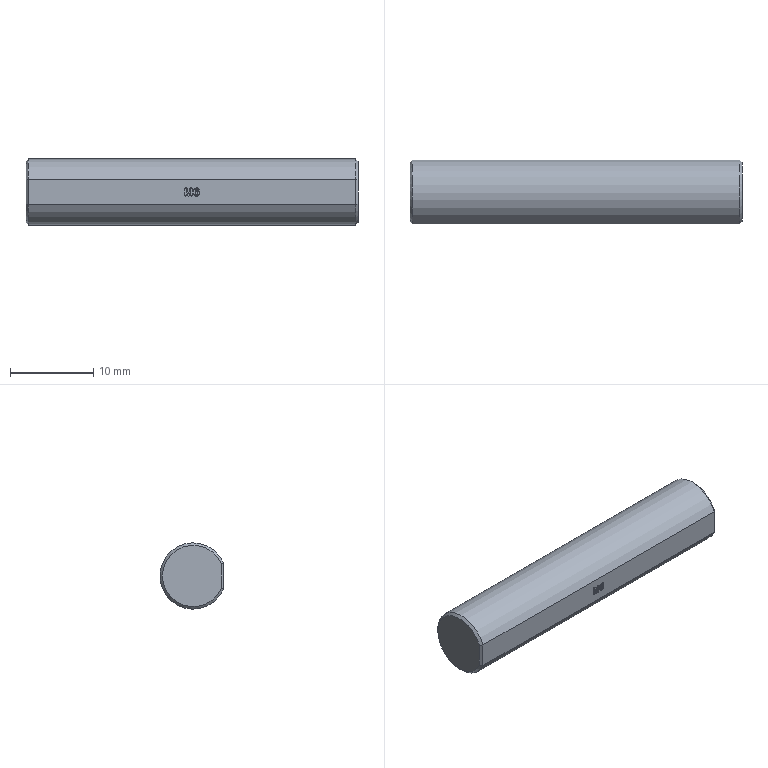Part | NX | features BREP 2, solid 2, SUBTRACT 1 | 1 solid | 28 faces | box 40 x 7.7 x 8 mm | volume 1857 mm3 | plane 12 | spline 9 | cone 4 | cylinder 3 | commonest cylinder face diameters 3.2 x1 4 x1 8 x1
STEP:
#1=CARTESIAN_POINT('',(236.55,-283.7,226.002));
#2=VERTEX_POINT('',#1);
#3=CARTESIAN_POINT('',(236.375,-283.7,226.545));
#4=VERTEX_POINT('',#3);
#5=CARTESIAN_POINT('',(236.55,-283.7,226.002));
#6=CARTESIAN_POINT('',(236.615,-283.7,226.002));
#7=CARTESIAN_POINT('',(236.673,-283.7,226.016));
#8=CARTESIAN_POINT('',(236.775,-283.7,226.073));
#9=CARTESIAN_POINT('',(236.815,-283.7,226.113));
#10=CARTESIAN_POINT('',(236.872,-283.7,226.215));
#11=CARTESIAN_POINT('',(236.886,-283.7,226.272));
#12=CARTESIAN_POINT('',(236.886,-283.7,226.377));
#13=CARTESIAN_POINT('',(236.879,-283.7,226.418));
#14=CARTESIAN_POINT('',(236.85,-283.7,226.497));
#15=CARTESIAN_POINT('',(236.829,-283.7,226.531));
#16=CARTESIAN_POINT('',(236.776,-283.7,226.589));
#17=CARTESIAN_POINT('',(236.744,-283.7,226.611));
#18=CARTESIAN_POINT('',(236.673,-283.7,226.643));
#19=CARTESIAN_POINT('',(236.634,-283.7,226.651));
#20=CARTESIAN_POINT('',(236.548,-283.7,226.651));
#21=CARTESIAN_POINT('',(236.509,-283.7,226.642));
#22=CARTESIAN_POINT('',(236.438,-283.7,226.608));
#23=CARTESIAN_POINT('',(236.405,-283.7,226.581));
#24=CARTESIAN_POINT('',(236.375,-283.7,226.545));
#25=B_SPLINE_CURVE_WITH_KNOTS('',3,(#5,#6,#7,#8,#9,#10,#11,#12,#13,#14,#15,#16,#17,#18,#19,#20,#21,#22,#23,#24),.UNSPECIFIED.,.F.,.F.,(4,2,2,2,2,2,2,2,2,4),(0.,0.02844,0.05688,0.08532,0.1049,0.1245,0.144,0.1636,0.184,0.2044),.UNSPECIFIED.);
#26=EDGE_CURVE('',#2,#4,#25,.T.);
#27=ORIENTED_EDGE('',*,*,#26,.F.);
#28=CARTESIAN_POINT('',(236.686,-283.7,226.783));
#29=VERTEX_POINT('',#28);
#30=CARTESIAN_POINT('',(236.686,-283.7,226.783));
#31=CARTESIAN_POINT('',(236.694,-283.7,226.762));
#32=CARTESIAN_POINT('',(236.706,-283.7,226.746));
#33=CARTESIAN_POINT('',(236.738,-283.7,226.722));
#34=CARTESIAN_POINT('',(236.755,-283.7,226.716));
#35=CARTESIAN_POINT('',(236.795,-283.7,226.716));
#36=CARTESIAN_POINT('',(236.812,-283.7,226.724));
#37=CARTESIAN_POINT('',(236.84,-283.7,226.754));
#38=CARTESIAN_POINT('',(236.846,-283.7,226.77));
#39=CARTESIAN_POINT('',(236.846,-283.7,226.818));
#40=CARTESIAN_POINT('',(236.836,-283.7,226.85));
#41=CARTESIAN_POINT('',(236.792,-283.7,226.915));
#42=CARTESIAN_POINT('',(236.759,-283.7,226.943));
#43=CARTESIAN_POINT('',(236.673,-283.7,226.987));
#44=CARTESIAN_POINT('',(236.623,-283.7,226.998));
#45=CARTESIAN_POINT('',(236.507,-283.7,226.998));
#46=CARTESIAN_POINT('',(236.455,-283.7,226.987));
#47=CARTESIAN_POINT('',(236.363,-283.7,226.943));
#48=CARTESIAN_POINT('',(236.324,-283.7,226.91));
#49=CARTESIAN_POINT('',(236.259,-283.7,226.823));
#50=CARTESIAN_POINT('',(236.234,-283.7,226.769));
#51=CARTESIAN_POINT('',(236.2,-283.7,226.637));
#52=CARTESIAN_POINT('',(236.191,-283.7,226.562));
#53=CARTESIAN_POINT('',(236.191,-283.7,226.375));
#54=CARTESIAN_POINT('',(236.205,-283.7,226.288));
#55=CARTESIAN_POINT('',(236.262,-283.7,226.146));
#56=CARTESIAN_POINT('',(236.304,-283.7,226.093));
#57=CARTESIAN_POINT('',(236.412,-283.7,226.02));
#58=CARTESIAN_POINT('',(236.476,-283.7,226.002));
#59=CARTESIAN_POINT('',(236.55,-283.7,226.002));
#60=B_SPLINE_CURVE_WITH_KNOTS('',3,(#30,#31,#32,#33,#34,#35,#36,#37,#38,#39,#40,#41,#42,#43,#44,#45,#46,#47,#48,#49,#50,#51,#52,#53,#54,#55,#56,#57,#58,#59),.UNSPECIFIED.,.F.,.F.,(4,2,2,2,2,2,2,2,2,2,2,2,2,2,4),(0.3727,0.3977,0.4227,0.4513,0.4798,0.5272,0.5745,0.6219,0.6711,0.7203,0.7695,0.8188,0.8792,0.9396,1.),.UNSPECIFIED.);
#61=EDGE_CURVE('',#29,#2,#60,.T.);
#62=ORIENTED_EDGE('',*,*,#61,.F.);
#63=CARTESIAN_POINT('',(236.432,-283.7,226.796));
#64=VERTEX_POINT('',#63);
#65=CARTESIAN_POINT('',(236.432,-283.7,226.796));
#66=CARTESIAN_POINT('',(236.448,-283.7,226.819));
#67=CARTESIAN_POINT('',(236.468,-283.7,226.837));
#68=CARTESIAN_POINT('',(236.514,-283.7,226.864));
#69=CARTESIAN_POINT('',(236.537,-283.7,226.871));
#70=CARTESIAN_POINT('',(236.59,-283.7,226.871));
#71=CARTESIAN_POINT('',(236.616,-283.7,226.863));
#72=CARTESIAN_POINT('',(236.66,-283.7,226.831));
#73=CARTESIAN_POINT('',(236.676,-283.7,226.809));
#74=CARTESIAN_POINT('',(236.686,-283.7,226.783));
#75=B_SPLINE_CURVE_WITH_KNOTS('',3,(#65,#66,#67,#68,#69,#70,#71,#72,#73,#74),.UNSPECIFIED.,.F.,.F.,(4,2,2,2,4),(0.2569,0.2827,0.3085,0.3406,0.3727),.UNSPECIFIED.);
#76=EDGE_CURVE('',#64,#29,#75,.T.);
#77=ORIENTED_EDGE('',*,*,#76,.F.);
#78=CARTESIAN_POINT('',(236.375,-283.7,226.545));
#79=CARTESIAN_POINT('',(236.381,-283.7,226.666));
#80=CARTESIAN_POINT('',(236.4,-283.7,226.749));
#81=CARTESIAN_POINT('',(236.432,-283.7,226.796));
#82=B_SPLINE_CURVE_WITH_KNOTS('',3,(#78,#79,#80,#81),.UNSPECIFIED.,.F.,.F.,(4,4),(0.2044,0.2569),.PIECEWISE_BEZIER_KNOTS.);
#83=EDGE_CURVE('',#4,#64,#82,.T.);
#84=ORIENTED_EDGE('',*,*,#83,.F.);
#85=EDGE_LOOP('',(#27,#62,#77,#84));
#86=FACE_BOUND('',#85,.T.);
#87=CARTESIAN_POINT('',(255.7,-283.7,228.02));
#88=VERTEX_POINT('',#87);
#89=CARTESIAN_POINT('',(216.3,-283.7,228.02));
#90=VERTEX_POINT('',#89);
#91=CARTESIAN_POINT('',(216.,-283.7,228.02));
#92=DIRECTION('',(1.,0.,0.));
#93=VECTOR('',#92,1000.);
#94=LINE('',#91,#93);
#95=EDGE_CURVE('',#88,#90,#94,.F.);
#96=ORIENTED_EDGE('',*,*,#95,.T.);
#97=CARTESIAN_POINT('',(216.3,-283.7,224.98));
#98=VERTEX_POINT('',#97);
#99=CARTESIAN_POINT('',(216.3,-283.7,224.98));
#100=DIRECTION('',(0.,0.,-1.));
#101=VECTOR('',#100,1000.);
#102=LINE('',#99,#101);
#103=EDGE_CURVE('',#90,#98,#102,.T.);
#104=ORIENTED_EDGE('',*,*,#103,.T.);
#105=CARTESIAN_POINT('',(255.7,-283.7,224.98));
#106=VERTEX_POINT('',#105);
#107=CARTESIAN_POINT('',(216.,-283.7,224.98));
#108=DIRECTION('',(1.,0.,0.));
#109=VECTOR('',#108,1000.);
#110=LINE('',#107,#109);
#111=EDGE_CURVE('',#98,#106,#110,.T.);
#112=ORIENTED_EDGE('',*,*,#111,.T.);
#113=CARTESIAN_POINT('',(255.7,-283.7,228.02));
#114=DIRECTION('',(0.,0.,1.));
#115=VECTOR('',#114,1000.);
#116=LINE('',#113,#115);
#117=EDGE_CURVE('',#106,#88,#116,.T.);
#118=ORIENTED_EDGE('',*,*,#117,.T.);
#119=EDGE_LOOP('',(#96,#104,#112,#118));
#120=FACE_BOUND('',#119,.T.);
#121=CARTESIAN_POINT('',(235.203,-283.7,226.005));
#122=VERTEX_POINT('',#121);
#123=CARTESIAN_POINT('',(235.294,-283.7,226.783));
#124=VERTEX_POINT('',#123);
#125=CARTESIAN_POINT('',(235.203,-283.7,226.005));
#126=CARTESIAN_POINT('',(235.231,-283.7,226.005));
#127=CARTESIAN_POINT('',(235.252,-283.7,226.014));
#128=CARTESIAN_POINT('',(235.285,-283.7,226.051));
#129=CARTESIAN_POINT('',(235.294,-283.7,226.079));
#130=CARTESIAN_POINT('',(235.294,-283.7,226.338));
#131=CARTESIAN_POINT('',(235.294,-283.7,226.561));
#132=CARTESIAN_POINT('',(235.294,-283.7,226.783));
#133=B_SPLINE_CURVE_WITH_KNOTS('',3,(#125,#126,#127,#128,#129,#130,#131,#132),.UNSPECIFIED.,.F.,.F.,(4,2,2,4),(0.,0.01767,0.03533,0.1418),.UNSPECIFIED.);
#134=EDGE_CURVE('',#122,#124,#133,.T.);
#135=ORIENTED_EDGE('',*,*,#134,.F.);
#136=CARTESIAN_POINT('',(235.439,-283.7,226.859));
#137=VERTEX_POINT('',#136);
#138=CARTESIAN_POINT('',(235.439,-283.7,226.859));
#139=CARTESIAN_POINT('',(235.429,-283.7,226.898));
#140=CARTESIAN_POINT('',(235.42,-283.7,226.925));
#141=CARTESIAN_POINT('',(235.404,-283.7,226.96));
#142=CARTESIAN_POINT('',(235.392,-283.7,226.972));
#143=CARTESIAN_POINT('',(235.359,-283.7,226.985));
#144=CARTESIAN_POINT('',(235.333,-283.7,226.988));
#145=CARTESIAN_POINT('',(235.276,-283.7,226.988));
#146=CARTESIAN_POINT('',(235.256,-283.7,226.988));
#147=CARTESIAN_POINT('',(235.198,-283.7,226.988));
#148=CARTESIAN_POINT('',(235.169,-283.7,226.981));
#149=CARTESIAN_POINT('',(235.125,-283.7,226.951));
#150=CARTESIAN_POINT('',(235.114,-283.7,226.923));
#151=CARTESIAN_POINT('',(235.114,-283.7,226.626));
#152=CARTESIAN_POINT('',(235.114,-283.7,226.371));
#153=CARTESIAN_POINT('',(235.114,-283.7,226.079));
#154=CARTESIAN_POINT('',(235.122,-283.7,226.051));
#155=CARTESIAN_POINT('',(235.155,-283.7,226.014));
#156=CARTESIAN_POINT('',(235.177,-283.7,226.005));
#157=CARTESIAN_POINT('',(235.203,-283.7,226.005));
#158=B_SPLINE_CURVE_WITH_KNOTS('',3,(#138,#139,#140,#141,#142,#143,#144,#145,#146,#147,#148,#149,#150,#151,#152,#153,#154,#155,#156,#157),.UNSPECIFIED.,.F.,.F.,(4,2,2,2,2,2,2,2,2,4),(0.8075,0.8217,0.8358,0.85,0.8578,0.8723,0.8868,0.9743,0.9872,1.),.UNSPECIFIED.);
#159=EDGE_CURVE('',#137,#122,#158,.T.);
#160=ORIENTED_EDGE('',*,*,#159,.F.);
#161=CARTESIAN_POINT('',(235.58,-283.7,226.33));
#162=VERTEX_POINT('',#161);
#163=CARTESIAN_POINT('',(233.874,-283.7,232.761));
#164=DIRECTION('',(-0.2564,0.,0.9666));
#165=VECTOR('',#164,1000.);
#166=LINE('',#163,#165);
#167=EDGE_CURVE('',#162,#137,#166,.T.);
#168=ORIENTED_EDGE('',*,*,#167,.F.);
#169=CARTESIAN_POINT('',(235.72,-283.7,226.859));
#170=VERTEX_POINT('',#169);
#171=CARTESIAN_POINT('',(234.712,-283.7,223.057));
#172=DIRECTION('',(-0.2564,0.,-0.9666));
#173=VECTOR('',#172,1000.);
#174=LINE('',#171,#173);
#175=EDGE_CURVE('',#170,#162,#174,.T.);
#176=ORIENTED_EDGE('',*,*,#175,.F.);
#177=CARTESIAN_POINT('',(235.866,-283.7,226.783));
#178=VERTEX_POINT('',#177);
#179=CARTESIAN_POINT('',(235.866,-283.7,226.783));
#180=CARTESIAN_POINT('',(235.866,-283.7,226.561));
#181=CARTESIAN_POINT('',(235.866,-283.7,226.338));
#182=CARTESIAN_POINT('',(235.866,-283.7,226.079));
#183=CARTESIAN_POINT('',(235.874,-283.7,226.051));
#184=CARTESIAN_POINT('',(235.908,-283.7,226.014));
#185=CARTESIAN_POINT('',(235.929,-283.7,226.005));
#186=CARTESIAN_POINT('',(235.982,-283.7,226.005));
#187=CARTESIAN_POINT('',(236.005,-283.7,226.014));
#188=CARTESIAN_POINT('',(236.038,-283.7,226.051));
#189=CARTESIAN_POINT('',(236.046,-283.7,226.079));
#190=CARTESIAN_POINT('',(236.046,-283.7,226.371));
#191=CARTESIAN_POINT('',(236.046,-283.7,226.626));
#192=CARTESIAN_POINT('',(236.046,-283.7,226.923));
#193=CARTESIAN_POINT('',(236.035,-283.7,226.951));
#194=CARTESIAN_POINT('',(235.991,-283.7,226.981));
#195=CARTESIAN_POINT('',(235.961,-283.7,226.988));
#196=CARTESIAN_POINT('',(235.904,-283.7,226.988));
#197=CARTESIAN_POINT('',(235.883,-283.7,226.988));
#198=CARTESIAN_POINT('',(235.827,-283.7,226.988));
#199=CARTESIAN_POINT('',(235.8,-283.7,226.985));
#200=CARTESIAN_POINT('',(235.767,-283.7,226.972));
#201=CARTESIAN_POINT('',(235.755,-283.7,226.96));
#202=CARTESIAN_POINT('',(235.739,-283.7,226.925));
#203=CARTESIAN_POINT('',(235.73,-283.7,226.898));
#204=CARTESIAN_POINT('',(235.72,-283.7,226.859));
#205=B_SPLINE_CURVE_WITH_KNOTS('',3,(#179,#180,#181,#182,#183,#184,#185,#186,#187,#188,#189,#190,#191,#192,#193,#194,#195,#196,#197,#198,#199,#200,#201,#202,#203,#204),.UNSPECIFIED.,.F.,.F.,(4,2,2,2,2,2,2,2,2,2,2,2,4),(0.3909,0.4624,0.4743,0.4862,0.4988,0.5115,0.599,0.6135,0.628,0.6359,0.65,0.6642,0.6783),.UNSPECIFIED.);
#206=EDGE_CURVE('',#178,#170,#205,.T.);
#207=ORIENTED_EDGE('',*,*,#206,.F.);
#208=CARTESIAN_POINT('',(235.711,-283.7,226.167));
#209=VERTEX_POINT('',#208);
#210=CARTESIAN_POINT('',(234.976,-283.7,223.245));
#211=DIRECTION('',(0.244,0.,0.9698));
#212=VECTOR('',#211,1000.);
#213=LINE('',#210,#212);
#214=EDGE_CURVE('',#209,#178,#213,.T.);
#215=ORIENTED_EDGE('',*,*,#214,.F.);
#216=CARTESIAN_POINT('',(235.449,-283.7,226.167));
#217=VERTEX_POINT('',#216);
#218=CARTESIAN_POINT('',(235.449,-283.7,226.167));
#219=CARTESIAN_POINT('',(235.454,-283.7,226.147));
#220=CARTESIAN_POINT('',(235.459,-283.7,226.128));
#221=CARTESIAN_POINT('',(235.469,-283.7,226.09));
#222=CARTESIAN_POINT('',(235.476,-283.7,226.073));
#223=CARTESIAN_POINT('',(235.494,-283.7,226.043));
#224=CARTESIAN_POINT('',(235.506,-283.7,226.03));
#225=CARTESIAN_POINT('',(235.538,-283.7,226.01));
#226=CARTESIAN_POINT('',(235.557,-283.7,226.005));
#227=CARTESIAN_POINT('',(235.61,-283.7,226.005));
#228=CARTESIAN_POINT('',(235.634,-283.7,226.013));
#229=CARTESIAN_POINT('',(235.668,-283.7,226.044));
#230=CARTESIAN_POINT('',(235.68,-283.7,226.061));
#231=CARTESIAN_POINT('',(235.693,-283.7,226.098));
#232=CARTESIAN_POINT('',(235.701,-283.7,226.127));
#233=CARTESIAN_POINT('',(235.711,-283.7,226.167));
#234=B_SPLINE_CURVE_WITH_KNOTS('',3,(#218,#219,#220,#221,#222,#223,#224,#225,#226,#227,#228,#229,#230,#231,#232,#233),.UNSPECIFIED.,.F.,.F.,(4,2,2,2,2,2,2,4),(0.243,0.253,0.263,0.273,0.283,0.2963,0.3096,0.3228),.UNSPECIFIED.);
#235=EDGE_CURVE('',#217,#209,#234,.T.);
#236=ORIENTED_EDGE('',*,*,#235,.F.);
#237=CARTESIAN_POINT('',(233.852,-283.7,232.512));
#238=DIRECTION('',(0.244,0.,-0.9698));
#239=VECTOR('',#238,1000.);
#240=LINE('',#237,#239);
#241=EDGE_CURVE('',#124,#217,#240,.T.);
#242=ORIENTED_EDGE('',*,*,#241,.F.);
#243=EDGE_LOOP('',(#135,#160,#168,#176,#207,#215,#236,#242));
#244=FACE_BOUND('',#243,.T.);
#245=CARTESIAN_POINT('',(216.,-283.7,228.02));
#246=DIRECTION('',(0.,-1.,0.));
#247=DIRECTION('',(-1.,0.,0.));
#248=AXIS2_PLACEMENT_3D('',#245,#246,#247);
#249=PLANE('',#248);
#250=ADVANCED_FACE('',(#86,#120,#244),#249,.T.);
#251=ORIENTED_EDGE('',*,*,#111,.F.);
#252=CARTESIAN_POINT('',(216.3,-280.,226.5));
#253=DIRECTION('',(1.,0.,0.));
#254=DIRECTION('',(0.,1.,0.));
#255=AXIS2_PLACEMENT_3D('',#252,#253,#254);
#256=CIRCLE('',#255,4.);
#257=EDGE_CURVE('',#98,#90,#256,.T.);
#258=ORIENTED_EDGE('',*,*,#257,.T.);
#259=ORIENTED_EDGE('',*,*,#95,.F.);
#260=CARTESIAN_POINT('',(255.7,-280.,226.5));
#261=DIRECTION('',(-1.,0.,0.));
#262=DIRECTION('',(0.,1.,0.));
#263=AXIS2_PLACEMENT_3D('',#260,#261,#262);
#264=CIRCLE('',#263,4.);
#265=EDGE_CURVE('',#88,#106,#264,.T.);
#266=ORIENTED_EDGE('',*,*,#265,.T.);
#267=EDGE_LOOP('',(#251,#258,#259,#266));
#268=FACE_BOUND('',#267,.T.);
#269=CARTESIAN_POINT('',(216.,-280.,226.5));
#270=DIRECTION('',(1.,0.,0.));
#271=DIRECTION('',(0.,-1.,0.));
#272=AXIS2_PLACEMENT_3D('',#269,#270,#271);
#273=CYLINDRICAL_SURFACE('',#272,4.);
#274=ADVANCED_FACE('',(#268),#273,.T.);
#275=CARTESIAN_POINT('',(216.,-283.4,227.959));
#276=VERTEX_POINT('',#275);
#277=CARTESIAN_POINT('',(216.,-283.4,225.041));
#278=VERTEX_POINT('',#277);
#279=CARTESIAN_POINT('',(216.,-280.,226.5));
#280=DIRECTION('',(-1.,0.,0.));
#281=DIRECTION('',(0.,1.,0.));
#282=AXIS2_PLACEMENT_3D('',#279,#280,#281);
#283=CIRCLE('',#282,3.7);
#284=EDGE_CURVE('',#276,#278,#283,.T.);
#285=ORIENTED_EDGE('',*,*,#284,.T.);
#286=CARTESIAN_POINT('',(216.,-283.4,228.02));
#287=DIRECTION('',(0.,0.,1.));
#288=VECTOR('',#287,1000.);
#289=LINE('',#286,#288);
#290=EDGE_CURVE('',#278,#276,#289,.T.);
#291=ORIENTED_EDGE('',*,*,#290,.T.);
#292=EDGE_LOOP('',(#285,#291));
#293=FACE_BOUND('',#292,.T.);
#294=CARTESIAN_POINT('',(216.,-280.,226.5));
#295=DIRECTION('',(1.,0.,0.));
#296=DIRECTION('',(0.,-1.,0.));
#297=AXIS2_PLACEMENT_3D('',#294,#295,#296);
#298=PLANE('',#297);
#299=ADVANCED_FACE('',(#293),#298,.F.);
#300=CARTESIAN_POINT('',(256.,-278.,226.5));
#301=VERTEX_POINT('',#300);
#302=CARTESIAN_POINT('',(256.,-280.,226.5));
#303=DIRECTION('',(1.,0.,0.));
#304=DIRECTION('',(0.,1.,0.));
#305=AXIS2_PLACEMENT_3D('',#302,#303,#304);
#306=CIRCLE('',#305,2.);
#307=EDGE_CURVE('',#301,#301,#306,.T.);
#308=ORIENTED_EDGE('',*,*,#307,.F.);
#309=EDGE_LOOP('',(#308));
#310=FACE_BOUND('',#309,.T.);
#311=CARTESIAN_POINT('',(256.,-283.4,227.959));
#312=VERTEX_POINT('',#311);
#313=CARTESIAN_POINT('',(256.,-283.4,225.041));
#314=VERTEX_POINT('',#313);
#315=CARTESIAN_POINT('',(256.,-283.4,226.5));
#316=DIRECTION('',(0.,0.,-1.));
#317=VECTOR('',#316,1000.);
#318=LINE('',#315,#317);
#319=EDGE_CURVE('',#312,#314,#318,.T.);
#320=ORIENTED_EDGE('',*,*,#319,.T.);
#321=CARTESIAN_POINT('',(256.,-280.,226.5));
#322=DIRECTION('',(1.,0.,0.));
#323=DIRECTION('',(0.,1.,0.));
#324=AXIS2_PLACEMENT_3D('',#321,#322,#323);
#325=CIRCLE('',#324,3.7);
#326=EDGE_CURVE('',#314,#312,#325,.T.);
#327=ORIENTED_EDGE('',*,*,#326,.T.);
#328=EDGE_LOOP('',(#320,#327));
#329=FACE_BOUND('',#328,.T.);
#330=CARTESIAN_POINT('',(256.,-280.,226.5));
#331=DIRECTION('',(1.,0.,0.));
#332=DIRECTION('',(0.,-1.,0.));
#333=AXIS2_PLACEMENT_3D('',#330,#331,#332);
#334=PLANE('',#333);
#335=ADVANCED_FACE('',(#310,#329),#334,.T.);
#336=CARTESIAN_POINT('',(216.,-283.4,225.041));
#337=CARTESIAN_POINT('',(216.1,-283.5,225.02));
#338=CARTESIAN_POINT('',(216.2,-283.6,225.));
#339=CARTESIAN_POINT('',(216.3,-283.7,224.98));
#340=B_SPLINE_CURVE_WITH_KNOTS('',3,(#336,#337,#338,#339),.UNSPECIFIED.,.F.,.F.,(4,4),(0.,1.),.PIECEWISE_BEZIER_KNOTS.);
#341=EDGE_CURVE('',#278,#98,#340,.T.);
#342=ORIENTED_EDGE('',*,*,#341,.F.);
#343=ORIENTED_EDGE('',*,*,#284,.F.);
#344=CARTESIAN_POINT('',(216.3,-283.7,228.02));
#345=CARTESIAN_POINT('',(216.2,-283.6,228.));
#346=CARTESIAN_POINT('',(216.1,-283.5,227.98));
#347=CARTESIAN_POINT('',(216.,-283.4,227.959));
#348=B_SPLINE_CURVE_WITH_KNOTS('',3,(#344,#345,#346,#347),.UNSPECIFIED.,.F.,.F.,(4,4),(0.,1.),.PIECEWISE_BEZIER_KNOTS.);
#349=EDGE_CURVE('',#90,#276,#348,.T.);
#350=ORIENTED_EDGE('',*,*,#349,.F.);
#351=ORIENTED_EDGE('',*,*,#257,.F.);
#352=EDGE_LOOP('',(#342,#343,#350,#351));
#353=FACE_BOUND('',#352,.T.);
#354=CARTESIAN_POINT('',(216.3,-280.,226.5));
#355=DIRECTION('',(1.,0.,0.));
#356=DIRECTION('',(0.,-1.,0.));
#357=AXIS2_PLACEMENT_3D('',#354,#355,#356);
#358=CONICAL_SURFACE('',#357,4.,0.7854);
#359=ADVANCED_FACE('',(#353),#358,.T.);
#360=ORIENTED_EDGE('',*,*,#349,.T.);
#361=ORIENTED_EDGE('',*,*,#290,.F.);
#362=ORIENTED_EDGE('',*,*,#341,.T.);
#363=ORIENTED_EDGE('',*,*,#103,.F.);
#364=EDGE_LOOP('',(#360,#361,#362,#363));
#365=FACE_BOUND('',#364,.T.);
#366=CARTESIAN_POINT('',(216.3,-283.7,228.02));
#367=DIRECTION('',(-0.7071,-0.7071,0.));
#368=DIRECTION('',(-0.7071,0.7071,0.));
#369=AXIS2_PLACEMENT_3D('',#366,#367,#368);
#370=PLANE('',#369);
#371=ADVANCED_FACE('',(#365),#370,.T.);
#372=CARTESIAN_POINT('',(255.7,-283.7,228.02));
#373=CARTESIAN_POINT('',(255.8,-283.6,228.));
#374=CARTESIAN_POINT('',(255.9,-283.5,227.98));
#375=CARTESIAN_POINT('',(256.,-283.4,227.959));
#376=B_SPLINE_CURVE_WITH_KNOTS('',3,(#372,#373,#374,#375),.UNSPECIFIED.,.F.,.F.,(4,4),(0.,1.),.PIECEWISE_BEZIER_KNOTS.);
#377=EDGE_CURVE('',#88,#312,#376,.T.);
#378=ORIENTED_EDGE('',*,*,#377,.F.);
#379=ORIENTED_EDGE('',*,*,#117,.F.);
#380=CARTESIAN_POINT('',(256.,-283.4,225.041));
#381=CARTESIAN_POINT('',(255.9,-283.5,225.02));
#382=CARTESIAN_POINT('',(255.8,-283.6,225.));
#383=CARTESIAN_POINT('',(255.7,-283.7,224.98));
#384=B_SPLINE_CURVE_WITH_KNOTS('',3,(#380,#381,#382,#383),.UNSPECIFIED.,.F.,.F.,(4,4),(0.,1.),.PIECEWISE_BEZIER_KNOTS.);
#385=EDGE_CURVE('',#314,#106,#384,.T.);
#386=ORIENTED_EDGE('',*,*,#385,.F.);
#387=ORIENTED_EDGE('',*,*,#319,.F.);
#388=EDGE_LOOP('',(#378,#379,#386,#387));
#389=FACE_BOUND('',#388,.T.);
#390=CARTESIAN_POINT('',(256.,-283.4,226.5));
#391=DIRECTION('',(-0.7071,0.7071,0.));
#392=DIRECTION('',(0.7071,0.7071,0.));
#393=AXIS2_PLACEMENT_3D('',#390,#391,#392);
#394=PLANE('',#393);
#395=ADVANCED_FACE('',(#389),#394,.F.);
#396=ORIENTED_EDGE('',*,*,#385,.T.);
#397=ORIENTED_EDGE('',*,*,#265,.F.);
#398=ORIENTED_EDGE('',*,*,#377,.T.);
#399=ORIENTED_EDGE('',*,*,#326,.F.);
#400=EDGE_LOOP('',(#396,#397,#398,#399));
#401=FACE_BOUND('',#400,.T.);
#402=CARTESIAN_POINT('',(256.,-280.,226.5));
#403=DIRECTION('',(-1.,0.,0.));
#404=DIRECTION('',(0.,1.,0.));
#405=AXIS2_PLACEMENT_3D('',#402,#403,#404);
#406=CONICAL_SURFACE('',#405,3.7,0.7854);
#407=ADVANCED_FACE('',(#401),#406,.T.);
#408=CARTESIAN_POINT('',(244.176,-280.,226.5));
#409=VERTEX_POINT('',#408);
#410=VERTEX_LOOP('',#409);
#411=FACE_BOUND('',#410,.T.);
#412=CARTESIAN_POINT('',(245.1,-278.4,226.5));
#413=VERTEX_POINT('',#412);
#414=CARTESIAN_POINT('',(245.1,-280.,226.5));
#415=DIRECTION('',(-1.,0.,0.));
#416=DIRECTION('',(0.,1.,0.));
#417=AXIS2_PLACEMENT_3D('',#414,#415,#416);
#418=CIRCLE('',#417,1.6);
#419=EDGE_CURVE('',#413,#413,#418,.T.);
#420=ORIENTED_EDGE('',*,*,#419,.F.);
#421=EDGE_LOOP('',(#420));
#422=FACE_BOUND('',#421,.T.);
#423=CARTESIAN_POINT('',(245.1,-280.,226.5));
#424=DIRECTION('',(1.,0.,0.));
#425=DIRECTION('',(0.,-1.,0.));
#426=AXIS2_PLACEMENT_3D('',#423,#424,#425);
#427=CONICAL_SURFACE('',#426,1.6,1.047);
#428=ADVANCED_FACE('',(#411,#422),#427,.F.);
#429=ORIENTED_EDGE('',*,*,#419,.T.);
#430=EDGE_LOOP('',(#429));
#431=FACE_BOUND('',#430,.T.);
#432=CARTESIAN_POINT('',(247.6,-278.4,226.5));
#433=VERTEX_POINT('',#432);
#434=CARTESIAN_POINT('',(247.6,-280.,226.5));
#435=DIRECTION('',(-1.,0.,0.));
#436=DIRECTION('',(0.,1.,0.));
#437=AXIS2_PLACEMENT_3D('',#434,#435,#436);
#438=CIRCLE('',#437,1.6);
#439=EDGE_CURVE('',#433,#433,#438,.T.);
#440=ORIENTED_EDGE('',*,*,#439,.F.);
#441=EDGE_LOOP('',(#440));
#442=FACE_BOUND('',#441,.T.);
#443=CARTESIAN_POINT('',(256.,-280.,226.5));
#444=DIRECTION('',(1.,0.,0.));
#445=DIRECTION('',(0.,-1.,0.));
#446=AXIS2_PLACEMENT_3D('',#443,#444,#445);
#447=CYLINDRICAL_SURFACE('',#446,1.6);
#448=ADVANCED_FACE('',(#431,#442),#447,.F.);
#449=ORIENTED_EDGE('',*,*,#439,.T.);
#450=EDGE_LOOP('',(#449));
#451=FACE_BOUND('',#450,.T.);
#452=CARTESIAN_POINT('',(248.,-278.,226.5));
#453=VERTEX_POINT('',#452);
#454=CARTESIAN_POINT('',(248.,-280.,226.5));
#455=DIRECTION('',(-1.,0.,0.));
#456=DIRECTION('',(0.,1.,0.));
#457=AXIS2_PLACEMENT_3D('',#454,#455,#456);
#458=CIRCLE('',#457,2.);
#459=EDGE_CURVE('',#453,#453,#458,.T.);
#460=ORIENTED_EDGE('',*,*,#459,.F.);
#461=EDGE_LOOP('',(#460));
#462=FACE_BOUND('',#461,.T.);
#463=CARTESIAN_POINT('',(248.,-280.,226.5));
#464=DIRECTION('',(1.,0.,0.));
#465=DIRECTION('',(0.,-1.,0.));
#466=AXIS2_PLACEMENT_3D('',#463,#464,#465);
#467=CONICAL_SURFACE('',#466,2.,0.7854);
#468=ADVANCED_FACE('',(#451,#462),#467,.F.);
#469=ORIENTED_EDGE('',*,*,#459,.T.);
#470=EDGE_LOOP('',(#469));
#471=FACE_BOUND('',#470,.T.);
#472=ORIENTED_EDGE('',*,*,#307,.T.);
#473=EDGE_LOOP('',(#472));
#474=FACE_BOUND('',#473,.T.);
#475=CARTESIAN_POINT('',(256.,-280.,226.5));
#476=DIRECTION('',(1.,0.,0.));
#477=DIRECTION('',(0.,-1.,0.));
#478=AXIS2_PLACEMENT_3D('',#475,#476,#477);
#479=CYLINDRICAL_SURFACE('',#478,2.);
#480=ADVANCED_FACE('',(#471,#474),#479,.F.);
#481=ORIENTED_EDGE('',*,*,#134,.T.);
#482=CARTESIAN_POINT('',(235.294,-283.5,226.783));
#483=VERTEX_POINT('',#482);
#484=CARTESIAN_POINT('',(235.294,-283.5,226.783));
#485=DIRECTION('',(0.,-1.,0.));
#486=VECTOR('',#485,1000.);
#487=LINE('',#484,#486);
#488=EDGE_CURVE('',#124,#483,#487,.F.);
#489=ORIENTED_EDGE('',*,*,#488,.T.);
#490=CARTESIAN_POINT('',(235.203,-283.5,226.005));
#491=VERTEX_POINT('',#490);
#492=CARTESIAN_POINT('',(235.203,-283.5,226.005));
#493=CARTESIAN_POINT('',(235.231,-283.5,226.005));
#494=CARTESIAN_POINT('',(235.252,-283.5,226.014));
#495=CARTESIAN_POINT('',(235.285,-283.5,226.051));
#496=CARTESIAN_POINT('',(235.294,-283.5,226.079));
#497=CARTESIAN_POINT('',(235.294,-283.5,226.338));
#498=CARTESIAN_POINT('',(235.294,-283.5,226.561));
#499=CARTESIAN_POINT('',(235.294,-283.5,226.783));
#500=B_SPLINE_CURVE_WITH_KNOTS('',3,(#492,#493,#494,#495,#496,#497,#498,#499),.UNSPECIFIED.,.F.,.F.,(4,2,2,4),(0.,0.01767,0.03533,0.1418),.UNSPECIFIED.);
#501=EDGE_CURVE('',#483,#491,#500,.F.);
#502=ORIENTED_EDGE('',*,*,#501,.T.);
#503=CARTESIAN_POINT('',(235.203,-283.5,226.005));
#504=DIRECTION('',(0.,-1.,0.));
#505=VECTOR('',#504,1000.);
#506=LINE('',#503,#505);
#507=EDGE_CURVE('',#122,#491,#506,.F.);
#508=ORIENTED_EDGE('',*,*,#507,.F.);
#509=EDGE_LOOP('',(#481,#489,#502,#508));
#510=FACE_BOUND('',#509,.T.);
#511=CARTESIAN_POINT('',(235.203,-283.5,226.005));
#512=CARTESIAN_POINT('',(235.203,-283.7,226.005));
#513=CARTESIAN_POINT('',(235.313,-283.5,226.005));
#514=CARTESIAN_POINT('',(235.313,-283.7,226.005));
#515=CARTESIAN_POINT('',(235.284,-283.5,226.357));
#516=CARTESIAN_POINT('',(235.284,-283.7,226.357));
#517=CARTESIAN_POINT('',(235.294,-283.5,226.635));
#518=CARTESIAN_POINT('',(235.294,-283.7,226.635));
#519=CARTESIAN_POINT('',(235.294,-283.5,226.783));
#520=CARTESIAN_POINT('',(235.294,-283.7,226.783));
#521=B_SPLINE_SURFACE_WITH_KNOTS('',3,1,((#511,#512),(#513,#514),(#515,#516),(#517,#518),(#519,#520)),.SURF_OF_LINEAR_EXTRUSION.,.F.,.F.,.F.,(4,1,4),(2,2),(0.,0.07088,0.1418),(0.,1.),.UNSPECIFIED.);
#522=ADVANCED_FACE('',(#510),#521,.F.);
#523=ORIENTED_EDGE('',*,*,#241,.T.);
#524=CARTESIAN_POINT('',(235.449,-283.5,226.167));
#525=VERTEX_POINT('',#524);
#526=CARTESIAN_POINT('',(235.449,-283.5,226.167));
#527=DIRECTION('',(0.,-1.,0.));
#528=VECTOR('',#527,1000.);
#529=LINE('',#526,#528);
#530=EDGE_CURVE('',#217,#525,#529,.F.);
#531=ORIENTED_EDGE('',*,*,#530,.T.);
#532=CARTESIAN_POINT('',(235.294,-283.5,226.783));
#533=CARTESIAN_POINT('',(235.345,-283.5,226.578));
#534=CARTESIAN_POINT('',(235.397,-283.5,226.373));
#535=CARTESIAN_POINT('',(235.449,-283.5,226.167));
#536=B_SPLINE_CURVE_WITH_KNOTS('',3,(#532,#533,#534,#535),.UNSPECIFIED.,.F.,.F.,(4,4),(0.1418,0.243),.PIECEWISE_BEZIER_KNOTS.);
#537=EDGE_CURVE('',#525,#483,#536,.F.);
#538=ORIENTED_EDGE('',*,*,#537,.T.);
#539=ORIENTED_EDGE('',*,*,#488,.F.);
#540=EDGE_LOOP('',(#523,#531,#538,#539));
#541=FACE_BOUND('',#540,.T.);
#542=CARTESIAN_POINT('',(235.294,-283.5,226.783));
#543=DIRECTION('',(-0.9698,0.,-0.244));
#544=DIRECTION('',(-0.244,0.,0.9698));
#545=AXIS2_PLACEMENT_3D('',#542,#543,#544);
#546=PLANE('',#545);
#547=ADVANCED_FACE('',(#541),#546,.F.);
#548=ORIENTED_EDGE('',*,*,#235,.T.);
#549=CARTESIAN_POINT('',(235.711,-283.5,226.167));
#550=VERTEX_POINT('',#549);
#551=CARTESIAN_POINT('',(235.711,-283.5,226.167));
#552=DIRECTION('',(0.,-1.,0.));
#553=VECTOR('',#552,1000.);
#554=LINE('',#551,#553);
#555=EDGE_CURVE('',#209,#550,#554,.F.);
#556=ORIENTED_EDGE('',*,*,#555,.T.);
#557=CARTESIAN_POINT('',(235.449,-283.5,226.167));
#558=CARTESIAN_POINT('',(235.454,-283.5,226.147));
#559=CARTESIAN_POINT('',(235.459,-283.5,226.128));
#560=CARTESIAN_POINT('',(235.469,-283.5,226.09));
#561=CARTESIAN_POINT('',(235.476,-283.5,226.073));
#562=CARTESIAN_POINT('',(235.494,-283.5,226.043));
#563=CARTESIAN_POINT('',(235.506,-283.5,226.03));
#564=CARTESIAN_POINT('',(235.538,-283.5,226.01));
#565=CARTESIAN_POINT('',(235.557,-283.5,226.005));
#566=CARTESIAN_POINT('',(235.61,-283.5,226.005));
#567=CARTESIAN_POINT('',(235.634,-283.5,226.013));
#568=CARTESIAN_POINT('',(235.668,-283.5,226.044));
#569=CARTESIAN_POINT('',(235.68,-283.5,226.061));
#570=CARTESIAN_POINT('',(235.693,-283.5,226.098));
#571=CARTESIAN_POINT('',(235.701,-283.5,226.127));
#572=CARTESIAN_POINT('',(235.711,-283.5,226.167));
#573=B_SPLINE_CURVE_WITH_KNOTS('',3,(#557,#558,#559,#560,#561,#562,#563,#564,#565,#566,#567,#568,#569,#570,#571,#572),.UNSPECIFIED.,.F.,.F.,(4,2,2,2,2,2,2,4),(0.243,0.253,0.263,0.273,0.283,0.2963,0.3096,0.3228),.UNSPECIFIED.);
#574=EDGE_CURVE('',#550,#525,#573,.F.);
#575=ORIENTED_EDGE('',*,*,#574,.T.);
#576=ORIENTED_EDGE('',*,*,#530,.F.);
#577=EDGE_LOOP('',(#548,#556,#575,#576));
#578=FACE_BOUND('',#577,.T.);
#579=CARTESIAN_POINT('',(235.449,-283.5,226.167));
#580=CARTESIAN_POINT('',(235.449,-283.7,226.167));
#581=CARTESIAN_POINT('',(235.491,-283.5,226.006));
#582=CARTESIAN_POINT('',(235.491,-283.7,226.006));
#583=CARTESIAN_POINT('',(235.65,-283.5,225.927));
#584=CARTESIAN_POINT('',(235.65,-283.7,225.927));
#585=CARTESIAN_POINT('',(235.711,-283.5,226.167));
#586=CARTESIAN_POINT('',(235.711,-283.7,226.167));
#587=B_SPLINE_SURFACE_WITH_KNOTS('',3,1,((#579,#580),(#581,#582),(#583,#584),(#585,#586)),.SURF_OF_LINEAR_EXTRUSION.,.F.,.F.,.F.,(4,4),(2,2),(0.243,0.3228),(0.,1.),.PIECEWISE_BEZIER_KNOTS.);
#588=ADVANCED_FACE('',(#578),#587,.F.);
#589=ORIENTED_EDGE('',*,*,#214,.T.);
#590=CARTESIAN_POINT('',(235.866,-283.5,226.783));
#591=VERTEX_POINT('',#590);
#592=CARTESIAN_POINT('',(235.866,-283.5,226.783));
#593=DIRECTION('',(0.,-1.,0.));
#594=VECTOR('',#593,1000.);
#595=LINE('',#592,#594);
#596=EDGE_CURVE('',#178,#591,#595,.F.);
#597=ORIENTED_EDGE('',*,*,#596,.T.);
#598=CARTESIAN_POINT('',(235.711,-283.5,226.167));
#599=CARTESIAN_POINT('',(235.763,-283.5,226.373));
#600=CARTESIAN_POINT('',(235.814,-283.5,226.578));
#601=CARTESIAN_POINT('',(235.866,-283.5,226.783));
#602=B_SPLINE_CURVE_WITH_KNOTS('',3,(#598,#599,#600,#601),.UNSPECIFIED.,.F.,.F.,(4,4),(0.3228,0.3909),.PIECEWISE_BEZIER_KNOTS.);
#603=EDGE_CURVE('',#591,#550,#602,.F.);
#604=ORIENTED_EDGE('',*,*,#603,.T.);
#605=ORIENTED_EDGE('',*,*,#555,.F.);
#606=EDGE_LOOP('',(#589,#597,#604,#605));
#607=FACE_BOUND('',#606,.T.);
#608=CARTESIAN_POINT('',(235.711,-283.5,226.167));
#609=DIRECTION('',(0.9698,0.,-0.244));
#610=DIRECTION('',(-0.244,0.,-0.9698));
#611=AXIS2_PLACEMENT_3D('',#608,#609,#610);
#612=PLANE('',#611);
#613=ADVANCED_FACE('',(#607),#612,.F.);
#614=ORIENTED_EDGE('',*,*,#206,.T.);
#615=CARTESIAN_POINT('',(235.72,-283.5,226.859));
#616=VERTEX_POINT('',#615);
#617=CARTESIAN_POINT('',(235.72,-283.5,226.859));
#618=DIRECTION('',(0.,-1.,0.));
#619=VECTOR('',#618,1000.);
#620=LINE('',#617,#619);
#621=EDGE_CURVE('',#170,#616,#620,.F.);
#622=ORIENTED_EDGE('',*,*,#621,.T.);
#623=CARTESIAN_POINT('',(235.866,-283.5,226.783));
#624=CARTESIAN_POINT('',(235.866,-283.5,226.561));
#625=CARTESIAN_POINT('',(235.866,-283.5,226.338));
#626=CARTESIAN_POINT('',(235.866,-283.5,226.079));
#627=CARTESIAN_POINT('',(235.874,-283.5,226.051));
#628=CARTESIAN_POINT('',(235.908,-283.5,226.014));
#629=CARTESIAN_POINT('',(235.929,-283.5,226.005));
#630=CARTESIAN_POINT('',(235.982,-283.5,226.005));
#631=CARTESIAN_POINT('',(236.005,-283.5,226.014));
#632=CARTESIAN_POINT('',(236.038,-283.5,226.051));
#633=CARTESIAN_POINT('',(236.046,-283.5,226.079));
#634=CARTESIAN_POINT('',(236.046,-283.5,226.371));
#635=CARTESIAN_POINT('',(236.046,-283.5,226.626));
#636=CARTESIAN_POINT('',(236.046,-283.5,226.923));
#637=CARTESIAN_POINT('',(236.035,-283.5,226.951));
#638=CARTESIAN_POINT('',(235.991,-283.5,226.981));
#639=CARTESIAN_POINT('',(235.961,-283.5,226.988));
#640=CARTESIAN_POINT('',(235.904,-283.5,226.988));
#641=CARTESIAN_POINT('',(235.883,-283.5,226.988));
#642=CARTESIAN_POINT('',(235.827,-283.5,226.988));
#643=CARTESIAN_POINT('',(235.8,-283.5,226.985));
#644=CARTESIAN_POINT('',(235.767,-283.5,226.972));
#645=CARTESIAN_POINT('',(235.755,-283.5,226.96));
#646=CARTESIAN_POINT('',(235.739,-283.5,226.925));
#647=CARTESIAN_POINT('',(235.73,-283.5,226.898));
#648=CARTESIAN_POINT('',(235.72,-283.5,226.859));
#649=B_SPLINE_CURVE_WITH_KNOTS('',3,(#623,#624,#625,#626,#627,#628,#629,#630,#631,#632,#633,#634,#635,#636,#637,#638,#639,#640,#641,#642,#643,#644,#645,#646,#647,#648),.UNSPECIFIED.,.F.,.F.,(4,2,2,2,2,2,2,2,2,2,2,2,4),(0.3909,0.4624,0.4743,0.4862,0.4988,0.5115,0.599,0.6135,0.628,0.6359,0.65,0.6642,0.6783),.UNSPECIFIED.);
#650=EDGE_CURVE('',#616,#591,#649,.F.);
#651=ORIENTED_EDGE('',*,*,#650,.T.);
#652=ORIENTED_EDGE('',*,*,#596,.F.);
#653=EDGE_LOOP('',(#614,#622,#651,#652));
#654=FACE_BOUND('',#653,.T.);
#655=CARTESIAN_POINT('',(235.866,-283.5,226.783));
#656=CARTESIAN_POINT('',(235.866,-283.7,226.783));
#657=CARTESIAN_POINT('',(235.866,-283.5,226.671));
#658=CARTESIAN_POINT('',(235.866,-283.7,226.671));
#659=CARTESIAN_POINT('',(235.881,-283.5,226.461));
#660=CARTESIAN_POINT('',(235.881,-283.7,226.461));
#661=CARTESIAN_POINT('',(235.812,-283.5,226.067));
#662=CARTESIAN_POINT('',(235.812,-283.7,226.067));
#663=CARTESIAN_POINT('',(236.067,-283.5,225.947));
#664=CARTESIAN_POINT('',(236.067,-283.7,225.947));
#665=CARTESIAN_POINT('',(236.044,-283.5,226.336));
#666=CARTESIAN_POINT('',(236.044,-283.7,226.336));
#667=CARTESIAN_POINT('',(236.031,-283.5,226.613));
#668=CARTESIAN_POINT('',(236.031,-283.7,226.613));
#669=CARTESIAN_POINT('',(236.106,-283.5,227.));
#670=CARTESIAN_POINT('',(236.106,-283.7,227.));
#671=CARTESIAN_POINT('',(235.769,-283.5,226.994));
#672=CARTESIAN_POINT('',(235.769,-283.7,226.994));
#673=CARTESIAN_POINT('',(235.746,-283.5,226.957));
#674=CARTESIAN_POINT('',(235.746,-283.7,226.957));
#675=CARTESIAN_POINT('',(235.72,-283.5,226.859));
#676=CARTESIAN_POINT('',(235.72,-283.7,226.859));
#677=B_SPLINE_SURFACE_WITH_KNOTS('',3,1,((#655,#656),(#657,#658),(#659,#660),(#661,#662),(#663,#664),(#665,#666),(#667,#668),(#669,#670),(#671,#672),(#673,#674),(#675,#676)),.SURF_OF_LINEAR_EXTRUSION.,.F.,.F.,.F.,(4,1,1,1,1,1,1,1,4),(2,2),(0.3909,0.4268,0.4627,0.4987,0.5346,0.5705,0.6065,0.6424,0.6783),(0.,1.),.UNSPECIFIED.);
#678=ADVANCED_FACE('',(#654),#677,.F.);
#679=ORIENTED_EDGE('',*,*,#175,.T.);
#680=CARTESIAN_POINT('',(235.58,-283.5,226.33));
#681=VERTEX_POINT('',#680);
#682=CARTESIAN_POINT('',(235.58,-283.5,226.33));
#683=DIRECTION('',(0.,-1.,0.));
#684=VECTOR('',#683,1000.);
#685=LINE('',#682,#684);
#686=EDGE_CURVE('',#162,#681,#685,.F.);
#687=ORIENTED_EDGE('',*,*,#686,.T.);
#688=CARTESIAN_POINT('',(235.72,-283.5,226.859));
#689=CARTESIAN_POINT('',(235.673,-283.5,226.682));
#690=CARTESIAN_POINT('',(235.627,-283.5,226.506));
#691=CARTESIAN_POINT('',(235.58,-283.5,226.33));
#692=B_SPLINE_CURVE_WITH_KNOTS('',3,(#688,#689,#690,#691),.UNSPECIFIED.,.F.,.F.,(4,4),(0.6783,0.7429),.PIECEWISE_BEZIER_KNOTS.);
#693=EDGE_CURVE('',#681,#616,#692,.F.);
#694=ORIENTED_EDGE('',*,*,#693,.T.);
#695=ORIENTED_EDGE('',*,*,#621,.F.);
#696=EDGE_LOOP('',(#679,#687,#694,#695));
#697=FACE_BOUND('',#696,.T.);
#698=CARTESIAN_POINT('',(235.72,-283.5,226.859));
#699=DIRECTION('',(-0.9666,0.,0.2564));
#700=DIRECTION('',(0.2564,0.,0.9666));
#701=AXIS2_PLACEMENT_3D('',#698,#699,#700);
#702=PLANE('',#701);
#703=ADVANCED_FACE('',(#697),#702,.F.);
#704=ORIENTED_EDGE('',*,*,#167,.T.);
#705=CARTESIAN_POINT('',(235.439,-283.5,226.859));
#706=VERTEX_POINT('',#705);
#707=CARTESIAN_POINT('',(235.439,-283.5,226.859));
#708=DIRECTION('',(0.,-1.,0.));
#709=VECTOR('',#708,1000.);
#710=LINE('',#707,#709);
#711=EDGE_CURVE('',#137,#706,#710,.F.);
#712=ORIENTED_EDGE('',*,*,#711,.T.);
#713=CARTESIAN_POINT('',(235.58,-283.5,226.33));
#714=CARTESIAN_POINT('',(235.533,-283.5,226.506));
#715=CARTESIAN_POINT('',(235.486,-283.5,226.682));
#716=CARTESIAN_POINT('',(235.439,-283.5,226.859));
#717=B_SPLINE_CURVE_WITH_KNOTS('',3,(#713,#714,#715,#716),.UNSPECIFIED.,.F.,.F.,(4,4),(0.7429,0.8075),.PIECEWISE_BEZIER_KNOTS.);
#718=EDGE_CURVE('',#706,#681,#717,.F.);
#719=ORIENTED_EDGE('',*,*,#718,.T.);
#720=ORIENTED_EDGE('',*,*,#686,.F.);
#721=EDGE_LOOP('',(#704,#712,#719,#720));
#722=FACE_BOUND('',#721,.T.);
#723=CARTESIAN_POINT('',(235.58,-283.5,226.33));
#724=DIRECTION('',(0.9666,0.,0.2564));
#725=DIRECTION('',(0.2564,0.,-0.9666));
#726=AXIS2_PLACEMENT_3D('',#723,#724,#725);
#727=PLANE('',#726);
#728=ADVANCED_FACE('',(#722),#727,.F.);
#729=ORIENTED_EDGE('',*,*,#159,.T.);
#730=ORIENTED_EDGE('',*,*,#507,.T.);
#731=CARTESIAN_POINT('',(235.439,-283.5,226.859));
#732=CARTESIAN_POINT('',(235.429,-283.5,226.898));
#733=CARTESIAN_POINT('',(235.42,-283.5,226.925));
#734=CARTESIAN_POINT('',(235.404,-283.5,226.96));
#735=CARTESIAN_POINT('',(235.392,-283.5,226.972));
#736=CARTESIAN_POINT('',(235.359,-283.5,226.985));
#737=CARTESIAN_POINT('',(235.333,-283.5,226.988));
#738=CARTESIAN_POINT('',(235.276,-283.5,226.988));
#739=CARTESIAN_POINT('',(235.256,-283.5,226.988));
#740=CARTESIAN_POINT('',(235.198,-283.5,226.988));
#741=CARTESIAN_POINT('',(235.169,-283.5,226.981));
#742=CARTESIAN_POINT('',(235.125,-283.5,226.951));
#743=CARTESIAN_POINT('',(235.114,-283.5,226.923));
#744=CARTESIAN_POINT('',(235.114,-283.5,226.626));
#745=CARTESIAN_POINT('',(235.114,-283.5,226.371));
#746=CARTESIAN_POINT('',(235.114,-283.5,226.079));
#747=CARTESIAN_POINT('',(235.122,-283.5,226.051));
#748=CARTESIAN_POINT('',(235.155,-283.5,226.014));
#749=CARTESIAN_POINT('',(235.177,-283.5,226.005));
#750=CARTESIAN_POINT('',(235.203,-283.5,226.005));
#751=B_SPLINE_CURVE_WITH_KNOTS('',3,(#731,#732,#733,#734,#735,#736,#737,#738,#739,#740,#741,#742,#743,#744,#745,#746,#747,#748,#749,#750),.UNSPECIFIED.,.F.,.F.,(4,2,2,2,2,2,2,2,2,4),(0.8075,0.8217,0.8358,0.85,0.8578,0.8723,0.8868,0.9743,0.9872,1.),.UNSPECIFIED.);
#752=EDGE_CURVE('',#491,#706,#751,.F.);
#753=ORIENTED_EDGE('',*,*,#752,.T.);
#754=ORIENTED_EDGE('',*,*,#711,.F.);
#755=EDGE_LOOP('',(#729,#730,#753,#754));
#756=FACE_BOUND('',#755,.T.);
#757=CARTESIAN_POINT('',(235.439,-283.5,226.859));
#758=CARTESIAN_POINT('',(235.439,-283.7,226.859));
#759=CARTESIAN_POINT('',(235.422,-283.5,226.925));
#760=CARTESIAN_POINT('',(235.422,-283.7,226.925));
#761=CARTESIAN_POINT('',(235.414,-283.5,226.984));
#762=CARTESIAN_POINT('',(235.414,-283.7,226.984));
#763=CARTESIAN_POINT('',(235.253,-283.5,226.994));
#764=CARTESIAN_POINT('',(235.253,-283.7,226.994));
#765=CARTESIAN_POINT('',(235.09,-283.5,226.969));
#766=CARTESIAN_POINT('',(235.09,-283.7,226.969));
#767=CARTESIAN_POINT('',(235.127,-283.5,226.646));
#768=CARTESIAN_POINT('',(235.127,-283.7,226.646));
#769=CARTESIAN_POINT('',(235.113,-283.5,226.33));
#770=CARTESIAN_POINT('',(235.113,-283.7,226.33));
#771=CARTESIAN_POINT('',(235.104,-283.5,226.005));
#772=CARTESIAN_POINT('',(235.104,-283.7,226.005));
#773=CARTESIAN_POINT('',(235.203,-283.5,226.005));
#774=CARTESIAN_POINT('',(235.203,-283.7,226.005));
#775=B_SPLINE_SURFACE_WITH_KNOTS('',3,1,((#757,#758),(#759,#760),(#761,#762),(#763,#764),(#765,#766),(#767,#768),(#769,#770),(#771,#772),(#773,#774)),.SURF_OF_LINEAR_EXTRUSION.,.F.,.F.,.F.,(4,1,1,1,1,1,4),(2,2),(0.8075,0.8316,0.8557,0.8797,0.9038,0.9519,1.),(0.,1.),.UNSPECIFIED.);
#776=ADVANCED_FACE('',(#756),#775,.F.);
#777=ORIENTED_EDGE('',*,*,#501,.F.);
#778=ORIENTED_EDGE('',*,*,#537,.F.);
#779=ORIENTED_EDGE('',*,*,#574,.F.);
#780=ORIENTED_EDGE('',*,*,#603,.F.);
#781=ORIENTED_EDGE('',*,*,#650,.F.);
#782=ORIENTED_EDGE('',*,*,#693,.F.);
#783=ORIENTED_EDGE('',*,*,#718,.F.);
#784=ORIENTED_EDGE('',*,*,#752,.F.);
#785=EDGE_LOOP('',(#777,#778,#779,#780,#781,#782,#783,#784));
#786=FACE_BOUND('',#785,.T.);
#787=CARTESIAN_POINT('',(235.294,-283.5,226.339));
#788=DIRECTION('',(0.,1.,0.));
#789=DIRECTION('',(0.,0.,1.));
#790=AXIS2_PLACEMENT_3D('',#787,#788,#789);
#791=PLANE('',#790);
#792=ADVANCED_FACE('',(#786),#791,.F.);
#793=ORIENTED_EDGE('',*,*,#26,.T.);
#794=CARTESIAN_POINT('',(236.375,-283.5,226.545));
#795=VERTEX_POINT('',#794);
#796=CARTESIAN_POINT('',(236.375,-283.5,226.545));
#797=DIRECTION('',(0.,-1.,0.));
#798=VECTOR('',#797,1000.);
#799=LINE('',#796,#798);
#800=EDGE_CURVE('',#4,#795,#799,.F.);
#801=ORIENTED_EDGE('',*,*,#800,.T.);
#802=CARTESIAN_POINT('',(236.55,-283.5,226.002));
#803=VERTEX_POINT('',#802);
#804=CARTESIAN_POINT('',(236.55,-283.5,226.002));
#805=CARTESIAN_POINT('',(236.615,-283.5,226.002));
#806=CARTESIAN_POINT('',(236.673,-283.5,226.016));
#807=CARTESIAN_POINT('',(236.775,-283.5,226.073));
#808=CARTESIAN_POINT('',(236.815,-283.5,226.113));
#809=CARTESIAN_POINT('',(236.872,-283.5,226.215));
#810=CARTESIAN_POINT('',(236.886,-283.5,226.272));
#811=CARTESIAN_POINT('',(236.886,-283.5,226.377));
#812=CARTESIAN_POINT('',(236.879,-283.5,226.418));
#813=CARTESIAN_POINT('',(236.85,-283.5,226.497));
#814=CARTESIAN_POINT('',(236.829,-283.5,226.531));
#815=CARTESIAN_POINT('',(236.776,-283.5,226.589));
#816=CARTESIAN_POINT('',(236.744,-283.5,226.611));
#817=CARTESIAN_POINT('',(236.673,-283.5,226.643));
#818=CARTESIAN_POINT('',(236.634,-283.5,226.651));
#819=CARTESIAN_POINT('',(236.548,-283.5,226.651));
#820=CARTESIAN_POINT('',(236.509,-283.5,226.642));
#821=CARTESIAN_POINT('',(236.438,-283.5,226.608));
#822=CARTESIAN_POINT('',(236.405,-283.5,226.581));
#823=CARTESIAN_POINT('',(236.375,-283.5,226.545));
#824=B_SPLINE_CURVE_WITH_KNOTS('',3,(#804,#805,#806,#807,#808,#809,#810,#811,#812,#813,#814,#815,#816,#817,#818,#819,#820,#821,#822,#823),.UNSPECIFIED.,.F.,.F.,(4,2,2,2,2,2,2,2,2,4),(0.,0.02844,0.05688,0.08532,0.1049,0.1245,0.144,0.1636,0.184,0.2044),.UNSPECIFIED.);
#825=EDGE_CURVE('',#795,#803,#824,.F.);
#826=ORIENTED_EDGE('',*,*,#825,.T.);
#827=CARTESIAN_POINT('',(236.55,-283.5,226.002));
#828=DIRECTION('',(0.,-1.,0.));
#829=VECTOR('',#828,1000.);
#830=LINE('',#827,#829);
#831=EDGE_CURVE('',#2,#803,#830,.F.);
#832=ORIENTED_EDGE('',*,*,#831,.F.);
#833=EDGE_LOOP('',(#793,#801,#826,#832));
#834=FACE_BOUND('',#833,.T.);
#835=CARTESIAN_POINT('',(236.55,-283.5,226.002));
#836=CARTESIAN_POINT('',(236.55,-283.7,226.002));
#837=CARTESIAN_POINT('',(236.783,-283.5,226.002));
#838=CARTESIAN_POINT('',(236.783,-283.7,226.002));
#839=CARTESIAN_POINT('',(237.086,-283.5,226.519));
#840=CARTESIAN_POINT('',(237.086,-283.7,226.519));
#841=CARTESIAN_POINT('',(236.526,-283.5,226.725));
#842=CARTESIAN_POINT('',(236.526,-283.7,226.725));
#843=CARTESIAN_POINT('',(236.375,-283.5,226.545));
#844=CARTESIAN_POINT('',(236.375,-283.7,226.545));
#845=B_SPLINE_SURFACE_WITH_KNOTS('',3,1,((#835,#836),(#837,#838),(#839,#840),(#841,#842),(#843,#844)),.SURF_OF_LINEAR_EXTRUSION.,.F.,.F.,.F.,(4,1,4),(2,2),(0.,0.1022,0.2044),(0.,1.),.UNSPECIFIED.);
#846=ADVANCED_FACE('',(#834),#845,.F.);
#847=ORIENTED_EDGE('',*,*,#83,.T.);
#848=CARTESIAN_POINT('',(236.432,-283.5,226.796));
#849=VERTEX_POINT('',#848);
#850=CARTESIAN_POINT('',(236.432,-283.5,226.796));
#851=DIRECTION('',(0.,-1.,0.));
#852=VECTOR('',#851,1000.);
#853=LINE('',#850,#852);
#854=EDGE_CURVE('',#64,#849,#853,.F.);
#855=ORIENTED_EDGE('',*,*,#854,.T.);
#856=CARTESIAN_POINT('',(236.375,-283.5,226.545));
#857=CARTESIAN_POINT('',(236.381,-283.5,226.666));
#858=CARTESIAN_POINT('',(236.4,-283.5,226.749));
#859=CARTESIAN_POINT('',(236.432,-283.5,226.796));
#860=B_SPLINE_CURVE_WITH_KNOTS('',3,(#856,#857,#858,#859),.UNSPECIFIED.,.F.,.F.,(4,4),(0.2044,0.2569),.PIECEWISE_BEZIER_KNOTS.);
#861=EDGE_CURVE('',#849,#795,#860,.F.);
#862=ORIENTED_EDGE('',*,*,#861,.T.);
#863=ORIENTED_EDGE('',*,*,#800,.F.);
#864=EDGE_LOOP('',(#847,#855,#862,#863));
#865=FACE_BOUND('',#864,.T.);
#866=CARTESIAN_POINT('',(236.375,-283.5,226.545));
#867=CARTESIAN_POINT('',(236.375,-283.7,226.545));
#868=CARTESIAN_POINT('',(236.381,-283.5,226.666));
#869=CARTESIAN_POINT('',(236.381,-283.7,226.666));
#870=CARTESIAN_POINT('',(236.4,-283.5,226.749));
#871=CARTESIAN_POINT('',(236.4,-283.7,226.749));
#872=CARTESIAN_POINT('',(236.432,-283.5,226.796));
#873=CARTESIAN_POINT('',(236.432,-283.7,226.796));
#874=B_SPLINE_SURFACE_WITH_KNOTS('',3,1,((#866,#867),(#868,#869),(#870,#871),(#872,#873)),.SURF_OF_LINEAR_EXTRUSION.,.F.,.F.,.F.,(4,4),(2,2),(0.2044,0.2569),(0.,1.),.PIECEWISE_BEZIER_KNOTS.);
#875=ADVANCED_FACE('',(#865),#874,.F.);
#876=ORIENTED_EDGE('',*,*,#76,.T.);
#877=CARTESIAN_POINT('',(236.686,-283.5,226.783));
#878=VERTEX_POINT('',#877);
#879=CARTESIAN_POINT('',(236.686,-283.5,226.783));
#880=DIRECTION('',(0.,-1.,0.));
#881=VECTOR('',#880,1000.);
#882=LINE('',#879,#881);
#883=EDGE_CURVE('',#29,#878,#882,.F.);
#884=ORIENTED_EDGE('',*,*,#883,.T.);
#885=CARTESIAN_POINT('',(236.432,-283.5,226.796));
#886=CARTESIAN_POINT('',(236.448,-283.5,226.819));
#887=CARTESIAN_POINT('',(236.468,-283.5,226.837));
#888=CARTESIAN_POINT('',(236.514,-283.5,226.864));
#889=CARTESIAN_POINT('',(236.537,-283.5,226.871));
#890=CARTESIAN_POINT('',(236.59,-283.5,226.871));
#891=CARTESIAN_POINT('',(236.616,-283.5,226.863));
#892=CARTESIAN_POINT('',(236.66,-283.5,226.831));
#893=CARTESIAN_POINT('',(236.676,-283.5,226.809));
#894=CARTESIAN_POINT('',(236.686,-283.5,226.783));
#895=B_SPLINE_CURVE_WITH_KNOTS('',3,(#885,#886,#887,#888,#889,#890,#891,#892,#893,#894),.UNSPECIFIED.,.F.,.F.,(4,2,2,2,4),(0.2569,0.2827,0.3085,0.3406,0.3727),.UNSPECIFIED.);
#896=EDGE_CURVE('',#878,#849,#895,.F.);
#897=ORIENTED_EDGE('',*,*,#896,.T.);
#898=ORIENTED_EDGE('',*,*,#854,.F.);
#899=EDGE_LOOP('',(#876,#884,#897,#898));
#900=FACE_BOUND('',#899,.T.);
#901=CARTESIAN_POINT('',(236.432,-283.5,226.796));
#902=CARTESIAN_POINT('',(236.432,-283.7,226.796));
#903=CARTESIAN_POINT('',(236.504,-283.5,226.9));
#904=CARTESIAN_POINT('',(236.504,-283.7,226.9));
#905=CARTESIAN_POINT('',(236.65,-283.5,226.879));
#906=CARTESIAN_POINT('',(236.65,-283.7,226.879));
#907=CARTESIAN_POINT('',(236.686,-283.5,226.783));
#908=CARTESIAN_POINT('',(236.686,-283.7,226.783));
#909=B_SPLINE_SURFACE_WITH_KNOTS('',3,1,((#901,#902),(#903,#904),(#905,#906),(#907,#908)),.SURF_OF_LINEAR_EXTRUSION.,.F.,.F.,.F.,(4,4),(2,2),(0.2569,0.3727),(0.,1.),.PIECEWISE_BEZIER_KNOTS.);
#910=ADVANCED_FACE('',(#900),#909,.F.);
#911=ORIENTED_EDGE('',*,*,#61,.T.);
#912=ORIENTED_EDGE('',*,*,#831,.T.);
#913=CARTESIAN_POINT('',(236.686,-283.5,226.783));
#914=CARTESIAN_POINT('',(236.694,-283.5,226.762));
#915=CARTESIAN_POINT('',(236.706,-283.5,226.746));
#916=CARTESIAN_POINT('',(236.738,-283.5,226.722));
#917=CARTESIAN_POINT('',(236.755,-283.5,226.716));
#918=CARTESIAN_POINT('',(236.795,-283.5,226.716));
#919=CARTESIAN_POINT('',(236.812,-283.5,226.724));
#920=CARTESIAN_POINT('',(236.84,-283.5,226.754));
#921=CARTESIAN_POINT('',(236.846,-283.5,226.77));
#922=CARTESIAN_POINT('',(236.846,-283.5,226.818));
#923=CARTESIAN_POINT('',(236.836,-283.5,226.85));
#924=CARTESIAN_POINT('',(236.792,-283.5,226.915));
#925=CARTESIAN_POINT('',(236.759,-283.5,226.943));
#926=CARTESIAN_POINT('',(236.673,-283.5,226.987));
#927=CARTESIAN_POINT('',(236.623,-283.5,226.998));
#928=CARTESIAN_POINT('',(236.507,-283.5,226.998));
#929=CARTESIAN_POINT('',(236.455,-283.5,226.987));
#930=CARTESIAN_POINT('',(236.363,-283.5,226.943));
#931=CARTESIAN_POINT('',(236.324,-283.5,226.91));
#932=CARTESIAN_POINT('',(236.259,-283.5,226.823));
#933=CARTESIAN_POINT('',(236.234,-283.5,226.769));
#934=CARTESIAN_POINT('',(236.2,-283.5,226.637));
#935=CARTESIAN_POINT('',(236.191,-283.5,226.562));
#936=CARTESIAN_POINT('',(236.191,-283.5,226.375));
#937=CARTESIAN_POINT('',(236.205,-283.5,226.288));
#938=CARTESIAN_POINT('',(236.262,-283.5,226.146));
#939=CARTESIAN_POINT('',(236.304,-283.5,226.093));
#940=CARTESIAN_POINT('',(236.412,-283.5,226.02));
#941=CARTESIAN_POINT('',(236.476,-283.5,226.002));
#942=CARTESIAN_POINT('',(236.55,-283.5,226.002));
#943=B_SPLINE_CURVE_WITH_KNOTS('',3,(#913,#914,#915,#916,#917,#918,#919,#920,#921,#922,#923,#924,#925,#926,#927,#928,#929,#930,#931,#932,#933,#934,#935,#936,#937,#938,#939,#940,#941,#942),.UNSPECIFIED.,.F.,.F.,(4,2,2,2,2,2,2,2,2,2,2,2,2,2,4),(0.3727,0.3977,0.4227,0.4513,0.4798,0.5272,0.5745,0.6219,0.6711,0.7203,0.7695,0.8188,0.8792,0.9396,1.),.UNSPECIFIED.);
#944=EDGE_CURVE('',#803,#878,#943,.F.);
#945=ORIENTED_EDGE('',*,*,#944,.T.);
#946=ORIENTED_EDGE('',*,*,#883,.F.);
#947=EDGE_LOOP('',(#911,#912,#945,#946));
#948=FACE_BOUND('',#947,.T.);
#949=CARTESIAN_POINT('',(236.686,-283.5,226.783));
#950=CARTESIAN_POINT('',(236.686,-283.7,226.783));
#951=CARTESIAN_POINT('',(236.71,-283.5,226.718));
#952=CARTESIAN_POINT('',(236.71,-283.7,226.718));
#953=CARTESIAN_POINT('',(236.87,-283.5,226.7));
#954=CARTESIAN_POINT('',(236.87,-283.7,226.7));
#955=CARTESIAN_POINT('',(236.835,-283.5,226.972));
#956=CARTESIAN_POINT('',(236.835,-283.7,226.972));
#957=CARTESIAN_POINT('',(236.396,-283.5,227.043));
#958=CARTESIAN_POINT('',(236.396,-283.7,227.043));
#959=CARTESIAN_POINT('',(236.203,-283.5,226.755));
#960=CARTESIAN_POINT('',(236.203,-283.7,226.755));
#961=CARTESIAN_POINT('',(236.163,-283.5,226.197));
#962=CARTESIAN_POINT('',(236.163,-283.7,226.197));
#963=CARTESIAN_POINT('',(236.357,-283.5,226.002));
#964=CARTESIAN_POINT('',(236.357,-283.7,226.002));
#965=CARTESIAN_POINT('',(236.55,-283.5,226.002));
#966=CARTESIAN_POINT('',(236.55,-283.7,226.002));
#967=B_SPLINE_SURFACE_WITH_KNOTS('',3,1,((#949,#950),(#951,#952),(#953,#954),(#955,#956),(#957,#958),(#959,#960),(#961,#962),(#963,#964),(#965,#966)),.SURF_OF_LINEAR_EXTRUSION.,.F.,.F.,.F.,(4,1,1,1,1,1,4),(2,2),(0.3727,0.4511,0.5295,0.6864,0.7648,0.8432,1.),(0.,1.),.UNSPECIFIED.);
#968=ADVANCED_FACE('',(#948),#967,.F.);
#969=CARTESIAN_POINT('',(236.554,-283.7,226.133));
#970=VERTEX_POINT('',#969);
#971=CARTESIAN_POINT('',(236.554,-283.7,226.133));
#972=CARTESIAN_POINT('',(236.507,-283.7,226.133));
#973=CARTESIAN_POINT('',(236.468,-283.7,226.153));
#974=CARTESIAN_POINT('',(236.406,-283.7,226.232));
#975=CARTESIAN_POINT('',(236.391,-283.7,226.282));
#976=CARTESIAN_POINT('',(236.391,-283.7,226.379));
#977=CARTESIAN_POINT('',(236.399,-283.7,226.412));
#978=CARTESIAN_POINT('',(236.429,-283.7,226.467));
#979=CARTESIAN_POINT('',(236.449,-283.7,226.488));
#980=CARTESIAN_POINT('',(236.499,-283.7,226.517));
#981=CARTESIAN_POINT('',(236.526,-283.7,226.525));
#982=CARTESIAN_POINT('',(236.582,-283.7,226.525));
#983=CARTESIAN_POINT('',(236.608,-283.7,226.517));
#984=CARTESIAN_POINT('',(236.656,-283.7,226.486));
#985=CARTESIAN_POINT('',(236.675,-283.7,226.464));
#986=CARTESIAN_POINT('',(236.702,-283.7,226.406));
#987=CARTESIAN_POINT('',(236.709,-283.7,226.372));
#988=CARTESIAN_POINT('',(236.709,-283.7,226.272));
#989=CARTESIAN_POINT('',(236.694,-283.7,226.224));
#990=CARTESIAN_POINT('',(236.636,-283.7,226.151));
#991=CARTESIAN_POINT('',(236.599,-283.7,226.133));
#992=CARTESIAN_POINT('',(236.554,-283.7,226.133));
#993=B_SPLINE_CURVE_WITH_KNOTS('',3,(#971,#972,#973,#974,#975,#976,#977,#978,#979,#980,#981,#982,#983,#984,#985,#986,#987,#988,#989,#990,#991,#992),.UNSPECIFIED.,.T.,.F.,(1,3,2,2,2,2,2,2,2,2,2,3,1),(-0.124,0.,0.1291,0.2582,0.3386,0.4189,0.4993,0.5835,0.6677,0.7519,0.876,1.,1.129),.UNSPECIFIED.);
#994=EDGE_CURVE('',#970,#970,#993,.T.);
#995=ORIENTED_EDGE('',*,*,#994,.T.);
#996=EDGE_LOOP('',(#995));
#997=FACE_BOUND('',#996,.T.);
#998=CARTESIAN_POINT('',(236.554,-283.5,226.133));
#999=VERTEX_POINT('',#998);
#1000=CARTESIAN_POINT('',(236.554,-283.5,226.133));
#1001=CARTESIAN_POINT('',(236.507,-283.5,226.133));
#1002=CARTESIAN_POINT('',(236.468,-283.5,226.153));
#1003=CARTESIAN_POINT('',(236.406,-283.5,226.232));
#1004=CARTESIAN_POINT('',(236.391,-283.5,226.282));
#1005=CARTESIAN_POINT('',(236.391,-283.5,226.379));
#1006=CARTESIAN_POINT('',(236.399,-283.5,226.412));
#1007=CARTESIAN_POINT('',(236.429,-283.5,226.467));
#1008=CARTESIAN_POINT('',(236.449,-283.5,226.488));
#1009=CARTESIAN_POINT('',(236.499,-283.5,226.517));
#1010=CARTESIAN_POINT('',(236.526,-283.5,226.525));
#1011=CARTESIAN_POINT('',(236.582,-283.5,226.525));
#1012=CARTESIAN_POINT('',(236.608,-283.5,226.517));
#1013=CARTESIAN_POINT('',(236.656,-283.5,226.486));
#1014=CARTESIAN_POINT('',(236.675,-283.5,226.464));
#1015=CARTESIAN_POINT('',(236.702,-283.5,226.406));
#1016=CARTESIAN_POINT('',(236.709,-283.5,226.372));
#1017=CARTESIAN_POINT('',(236.709,-283.5,226.272));
#1018=CARTESIAN_POINT('',(236.694,-283.5,226.224));
#1019=CARTESIAN_POINT('',(236.636,-283.5,226.151));
#1020=CARTESIAN_POINT('',(236.599,-283.5,226.133));
#1021=CARTESIAN_POINT('',(236.554,-283.5,226.133));
#1022=B_SPLINE_CURVE_WITH_KNOTS('',3,(#1000,#1001,#1002,#1003,#1004,#1005,#1006,#1007,#1008,#1009,#1010,#1011,#1012,#1013,#1014,#1015,#1016,#1017,#1018,#1019,#1020,#1021),.UNSPECIFIED.,.T.,.F.,(1,3,2,2,2,2,2,2,2,2,2,3,1),(-0.124,0.,0.1291,0.2582,0.3386,0.4189,0.4993,0.5835,0.6677,0.7519,0.876,1.,1.129),.UNSPECIFIED.);
#1023=EDGE_CURVE('',#999,#999,#1022,.F.);
#1024=ORIENTED_EDGE('',*,*,#1023,.T.);
#1025=EDGE_LOOP('',(#1024));
#1026=FACE_BOUND('',#1025,.T.);
#1027=CARTESIAN_POINT('',(236.785,-283.5,226.339));
#1028=CARTESIAN_POINT('',(236.785,-283.7,226.339));
#1029=CARTESIAN_POINT('',(236.558,-283.5,226.031));
#1030=CARTESIAN_POINT('',(236.558,-283.7,226.031));
#1031=CARTESIAN_POINT('',(236.308,-283.5,226.333));
#1032=CARTESIAN_POINT('',(236.308,-283.7,226.333));
#1033=CARTESIAN_POINT('',(236.558,-283.5,226.619));
#1034=CARTESIAN_POINT('',(236.558,-283.7,226.619));
#1035=CARTESIAN_POINT('',(236.785,-283.5,226.339));
#1036=CARTESIAN_POINT('',(236.785,-283.7,226.339));
#1037=CARTESIAN_POINT('',(236.558,-283.5,226.031));
#1038=CARTESIAN_POINT('',(236.558,-283.7,226.031));
#1039=CARTESIAN_POINT('',(236.308,-283.5,226.333));
#1040=CARTESIAN_POINT('',(236.308,-283.7,226.333));
#1041=B_SPLINE_SURFACE_WITH_KNOTS('',3,1,((#1027,#1028),(#1029,#1030),(#1031,#1032),(#1033,#1034),(#1035,#1036),(#1037,#1038),(#1039,#1040)),.SURF_OF_LINEAR_EXTRUSION.,.T.,.F.,.F.,(1,1,1,1,1,1,1,1,1,1,1),(2,2),(-0.75,-0.5,-0.25,0.,0.25,0.5,0.75,1.,1.25,1.5,1.75),(0.,1.),.UNSPECIFIED.);
#1042=ADVANCED_FACE('',(#997,#1026),#1041,.F.);
#1043=ORIENTED_EDGE('',*,*,#825,.F.);
#1044=ORIENTED_EDGE('',*,*,#861,.F.);
#1045=ORIENTED_EDGE('',*,*,#896,.F.);
#1046=ORIENTED_EDGE('',*,*,#944,.F.);
#1047=EDGE_LOOP('',(#1043,#1044,#1045,#1046));
#1048=FACE_BOUND('',#1047,.T.);
#1049=ORIENTED_EDGE('',*,*,#1023,.F.);
#1050=EDGE_LOOP('',(#1049));
#1051=FACE_BOUND('',#1050,.T.);
#1052=CARTESIAN_POINT('',(236.87,-283.5,226.441));
#1053=DIRECTION('',(0.,1.,0.));
#1054=DIRECTION('',(0.,0.,1.));
#1055=AXIS2_PLACEMENT_3D('',#1052,#1053,#1054);
#1056=PLANE('',#1055);
#1057=ADVANCED_FACE('',(#1048,#1051),#1056,.F.);
#1058=ORIENTED_EDGE('',*,*,#994,.F.);
#1059=EDGE_LOOP('',(#1058));
#1060=FACE_BOUND('',#1059,.T.);
#1061=CARTESIAN_POINT('',(216.,-283.7,228.02));
#1062=DIRECTION('',(0.,-1.,0.));
#1063=DIRECTION('',(-1.,0.,0.));
#1064=AXIS2_PLACEMENT_3D('',#1061,#1062,#1063);
#1065=PLANE('',#1064);
#1066=ADVANCED_FACE('',(#1060),#1065,.T.);
#1067=CLOSED_SHELL('',(#250,#274,#299,#335,#359,#371,#395,#407,#428,#448,#468,#480,#522,#547,#588,#613,#678,#703,#728,#776,#792,#846,#875,#910,#968,#1042,#1057,#1066));
#1068=MANIFOLD_SOLID_BREP('',#1067);
#1069=(LENGTH_UNIT()NAMED_UNIT(*)SI_UNIT(.MILLI.,.METRE.));
#1070=UNCERTAINTY_MEASURE_WITH_UNIT(LENGTH_MEASURE(0.0508),#1069,'','');
#1071=(NAMED_UNIT(*)PLANE_ANGLE_UNIT()SI_UNIT($,.RADIAN.));
#1072=(NAMED_UNIT(*)SI_UNIT($,.STERADIAN.)SOLID_ANGLE_UNIT());
#1073=(GEOMETRIC_REPRESENTATION_CONTEXT(3)GLOBAL_UNCERTAINTY_ASSIGNED_CONTEXT((#1070))GLOBAL_UNIT_ASSIGNED_CONTEXT((#1069,#1071,#1072))REPRESENTATION_CONTEXT('',''));
#1074=ADVANCED_BREP_SHAPE_REPRESENTATION('',(#1068),#1073);